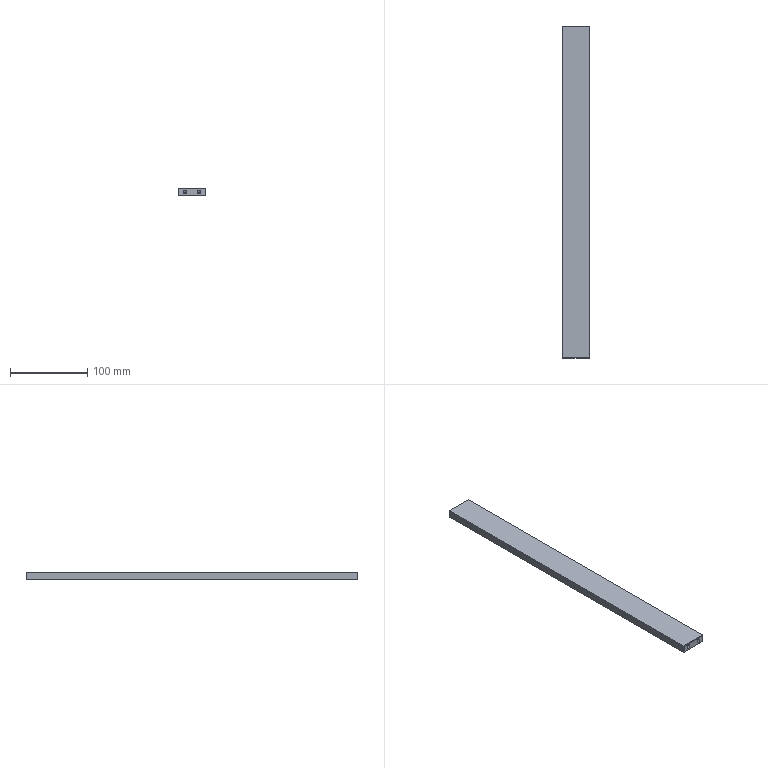Part | STEP file | Pino extrator - Torre - 1 cav | 1 solid | 18 faces | box 35 x 428.85 x 10 mm | volume 149085 mm3 | plane 10 | cylinder 4 | cone 4 | commonest cylinder face diameters 5 x4
STEP:
#1=CARTESIAN_POINT('',(0.,0.,0.));
#2=DIRECTION('',(0.,0.,1.));
#3=DIRECTION('',(1.,0.,0.));
#4=AXIS2_PLACEMENT_3D('',#1,#2,#3);
#5=CARTESIAN_POINT('',(-9.,25.,-2.5));
#6=VERTEX_POINT('',#5);
#7=CARTESIAN_POINT('',(-9.,0.,-2.5));
#8=VERTEX_POINT('',#7);
#9=CARTESIAN_POINT('',(-9.,0.,-2.5));
#10=DIRECTION('',(0.,-1.,0.));
#11=VECTOR('',#10,1.);
#12=LINE('',#9,#11);
#13=CARTESIAN_POINT('',(-9.,0.,0.));
#14=DIRECTION('',(0.,-1.,0.));
#15=DIRECTION('',(0.,0.,-1.));
#16=AXIS2_PLACEMENT_3D('',#13,#14,#15);
#17=CYLINDRICAL_SURFACE('',#16,2.5);
#18=CARTESIAN_POINT('',(6.283,0.));
#19=DIRECTION('',(0.,1.));
#20=VECTOR('',#19,1.);
#21=LINE('',#18,#20);
#22=(GEOMETRIC_REPRESENTATION_CONTEXT(2)PARAMETRIC_REPRESENTATION_CONTEXT()REPRESENTATION_CONTEXT('',''));
#23=DEFINITIONAL_REPRESENTATION('',(#21),#22);
#24=PCURVE('',#17,#23);
#25=CARTESIAN_POINT('',(-9.,0.,0.));
#26=DIRECTION('',(0.,-1.,0.));
#27=DIRECTION('',(0.,0.,-1.));
#28=AXIS2_PLACEMENT_3D('',#25,#26,#27);
#29=CYLINDRICAL_SURFACE('',#28,2.5);
#30=CARTESIAN_POINT('',(0.,0.));
#31=DIRECTION('',(0.,1.));
#32=VECTOR('',#31,1.);
#33=LINE('',#30,#32);
#34=(GEOMETRIC_REPRESENTATION_CONTEXT(2)PARAMETRIC_REPRESENTATION_CONTEXT()REPRESENTATION_CONTEXT('',''));
#35=DEFINITIONAL_REPRESENTATION('',(#33),#34);
#36=PCURVE('',#29,#35);
#37=SURFACE_CURVE('',#12,(#24,#36),.PCURVE_S1.);
#38=EDGE_CURVE('',#6,#8,#37,.T.);
#39=ORIENTED_EDGE('',*,*,#38,.T.);
#40=CARTESIAN_POINT('',(-9.,0.,2.5));
#41=VERTEX_POINT('',#40);
#42=CARTESIAN_POINT('',(-9.,0.,0.));
#43=DIRECTION('',(0.,-1.,0.));
#44=DIRECTION('',(0.,0.,-1.));
#45=AXIS2_PLACEMENT_3D('',#42,#43,#44);
#46=CIRCLE('',#45,2.5);
#47=CARTESIAN_POINT('',(0.,0.));
#48=DIRECTION('',(1.,0.));
#49=VECTOR('',#48,1.);
#50=LINE('',#47,#49);
#51=(GEOMETRIC_REPRESENTATION_CONTEXT(2)PARAMETRIC_REPRESENTATION_CONTEXT()REPRESENTATION_CONTEXT('',''));
#52=DEFINITIONAL_REPRESENTATION('',(#50),#51);
#53=PCURVE('',#17,#52);
#54=CARTESIAN_POINT('',(0.,0.,0.));
#55=DIRECTION('',(0.,-1.,0.));
#56=DIRECTION('',(0.,0.,-1.));
#57=AXIS2_PLACEMENT_3D('',#54,#55,#56);
#58=PLANE('',#57);
#59=CARTESIAN_POINT('',(0.,-9.));
#60=DIRECTION('',(1.,0.));
#61=AXIS2_PLACEMENT_2D('',#59,#60);
#62=CIRCLE('',#61,2.5);
#63=(GEOMETRIC_REPRESENTATION_CONTEXT(2)PARAMETRIC_REPRESENTATION_CONTEXT()REPRESENTATION_CONTEXT('',''));
#64=DEFINITIONAL_REPRESENTATION('',(#62),#63);
#65=PCURVE('',#58,#64);
#66=SURFACE_CURVE('',#46,(#53,#65),.PCURVE_S1.);
#67=EDGE_CURVE('',#41,#8,#66,.T.);
#68=ORIENTED_EDGE('',*,*,#67,.F.);
#69=CARTESIAN_POINT('',(-9.,25.,2.5));
#70=VERTEX_POINT('',#69);
#71=CARTESIAN_POINT('',(-9.,0.,2.5));
#72=DIRECTION('',(0.,-1.,0.));
#73=VECTOR('',#72,1.);
#74=LINE('',#71,#73);
#75=CARTESIAN_POINT('',(3.142,0.));
#76=DIRECTION('',(0.,1.));
#77=VECTOR('',#76,1.);
#78=LINE('',#75,#77);
#79=(GEOMETRIC_REPRESENTATION_CONTEXT(2)PARAMETRIC_REPRESENTATION_CONTEXT()REPRESENTATION_CONTEXT('',''));
#80=DEFINITIONAL_REPRESENTATION('',(#78),#79);
#81=PCURVE('',#17,#80);
#82=CARTESIAN_POINT('',(3.142,0.));
#83=DIRECTION('',(0.,1.));
#84=VECTOR('',#83,1.);
#85=LINE('',#82,#84);
#86=(GEOMETRIC_REPRESENTATION_CONTEXT(2)PARAMETRIC_REPRESENTATION_CONTEXT()REPRESENTATION_CONTEXT('',''));
#87=DEFINITIONAL_REPRESENTATION('',(#85),#86);
#88=PCURVE('',#29,#87);
#89=SURFACE_CURVE('',#74,(#81,#88),.PCURVE_S1.);
#90=EDGE_CURVE('',#70,#41,#89,.T.);
#91=ORIENTED_EDGE('',*,*,#90,.F.);
#92=CARTESIAN_POINT('',(-9.,25.,0.));
#93=DIRECTION('',(0.,-1.,0.));
#94=DIRECTION('',(0.,0.,-1.));
#95=AXIS2_PLACEMENT_3D('',#92,#93,#94);
#96=CIRCLE('',#95,2.5);
#97=CARTESIAN_POINT('',(0.,-25.));
#98=DIRECTION('',(1.,0.));
#99=VECTOR('',#98,1.);
#100=LINE('',#97,#99);
#101=(GEOMETRIC_REPRESENTATION_CONTEXT(2)PARAMETRIC_REPRESENTATION_CONTEXT()REPRESENTATION_CONTEXT('',''));
#102=DEFINITIONAL_REPRESENTATION('',(#100),#101);
#103=PCURVE('',#17,#102);
#104=CARTESIAN_POINT('',(-9.,25.,0.));
#105=DIRECTION('',(0.,-1.,0.));
#106=DIRECTION('',(0.,0.,-1.));
#107=AXIS2_PLACEMENT_3D('',#104,#105,#106);
#108=CONICAL_SURFACE('',#107,2.5,1.03);
#109=CARTESIAN_POINT('',(0.,0.));
#110=DIRECTION('',(1.,0.));
#111=VECTOR('',#110,1.);
#112=LINE('',#109,#111);
#113=(GEOMETRIC_REPRESENTATION_CONTEXT(2)PARAMETRIC_REPRESENTATION_CONTEXT()REPRESENTATION_CONTEXT('',''));
#114=DEFINITIONAL_REPRESENTATION('',(#112),#113);
#115=PCURVE('',#108,#114);
#116=SURFACE_CURVE('',#96,(#103,#115),.PCURVE_S1.);
#117=EDGE_CURVE('',#70,#6,#116,.T.);
#118=ORIENTED_EDGE('',*,*,#117,.T.);
#119=EDGE_LOOP('',(#39,#68,#91,#118));
#120=FACE_BOUND('',#119,.F.);
#121=ADVANCED_FACE('',(#120),#17,.F.);
#122=ORIENTED_EDGE('',*,*,#117,.F.);
#123=CARTESIAN_POINT('',(-9.,26.502,0.));
#124=VERTEX_POINT('',#123);
#125=CARTESIAN_POINT('',(-9.,25.,2.5));
#126=DIRECTION('',(0.,-0.515,0.8572));
#127=VECTOR('',#126,1.);
#128=LINE('',#125,#127);
#129=CARTESIAN_POINT('',(3.142,0.));
#130=DIRECTION('',(0.,1.));
#131=VECTOR('',#130,1.);
#132=LINE('',#129,#131);
#133=(GEOMETRIC_REPRESENTATION_CONTEXT(2)PARAMETRIC_REPRESENTATION_CONTEXT()REPRESENTATION_CONTEXT('',''));
#134=DEFINITIONAL_REPRESENTATION('',(#132),#133);
#135=PCURVE('',#108,#134);
#136=CARTESIAN_POINT('',(-9.,25.,0.));
#137=DIRECTION('',(0.,-1.,0.));
#138=DIRECTION('',(0.,0.,-1.));
#139=AXIS2_PLACEMENT_3D('',#136,#137,#138);
#140=CONICAL_SURFACE('',#139,2.5,1.03);
#141=CARTESIAN_POINT('',(3.142,0.));
#142=DIRECTION('',(0.,1.));
#143=VECTOR('',#142,1.);
#144=LINE('',#141,#143);
#145=(GEOMETRIC_REPRESENTATION_CONTEXT(2)PARAMETRIC_REPRESENTATION_CONTEXT()REPRESENTATION_CONTEXT('',''));
#146=DEFINITIONAL_REPRESENTATION('',(#144),#145);
#147=PCURVE('',#140,#146);
#148=SURFACE_CURVE('',#128,(#135,#147),.PCURVE_S1.);
#149=EDGE_CURVE('',#124,#70,#148,.T.);
#150=ORIENTED_EDGE('',*,*,#149,.F.);
#151=CARTESIAN_POINT('',(-9.,25.,-2.5));
#152=DIRECTION('',(0.,-0.515,-0.8572));
#153=VECTOR('',#152,1.);
#154=LINE('',#151,#153);
#155=CARTESIAN_POINT('',(6.283,0.));
#156=DIRECTION('',(0.,1.));
#157=VECTOR('',#156,1.);
#158=LINE('',#155,#157);
#159=(GEOMETRIC_REPRESENTATION_CONTEXT(2)PARAMETRIC_REPRESENTATION_CONTEXT()REPRESENTATION_CONTEXT('',''));
#160=DEFINITIONAL_REPRESENTATION('',(#158),#159);
#161=PCURVE('',#108,#160);
#162=CARTESIAN_POINT('',(0.,0.));
#163=DIRECTION('',(0.,1.));
#164=VECTOR('',#163,1.);
#165=LINE('',#162,#164);
#166=(GEOMETRIC_REPRESENTATION_CONTEXT(2)PARAMETRIC_REPRESENTATION_CONTEXT()REPRESENTATION_CONTEXT('',''));
#167=DEFINITIONAL_REPRESENTATION('',(#165),#166);
#168=PCURVE('',#140,#167);
#169=SURFACE_CURVE('',#154,(#161,#168),.PCURVE_S1.);
#170=EDGE_CURVE('',#124,#6,#169,.T.);
#171=ORIENTED_EDGE('',*,*,#170,.T.);
#172=EDGE_LOOP('',(#122,#150,#171));
#173=FACE_BOUND('',#172,.F.);
#174=ADVANCED_FACE('',(#173),#108,.F.);
#175=CARTESIAN_POINT('',(9.,25.,-2.5));
#176=VERTEX_POINT('',#175);
#177=CARTESIAN_POINT('',(9.,0.,-2.5));
#178=VERTEX_POINT('',#177);
#179=CARTESIAN_POINT('',(9.,0.,-2.5));
#180=DIRECTION('',(0.,-1.,0.));
#181=VECTOR('',#180,1.);
#182=LINE('',#179,#181);
#183=CARTESIAN_POINT('',(9.,0.,0.));
#184=DIRECTION('',(0.,-1.,0.));
#185=DIRECTION('',(0.,0.,-1.));
#186=AXIS2_PLACEMENT_3D('',#183,#184,#185);
#187=CYLINDRICAL_SURFACE('',#186,2.5);
#188=CARTESIAN_POINT('',(6.283,0.));
#189=DIRECTION('',(0.,1.));
#190=VECTOR('',#189,1.);
#191=LINE('',#188,#190);
#192=(GEOMETRIC_REPRESENTATION_CONTEXT(2)PARAMETRIC_REPRESENTATION_CONTEXT()REPRESENTATION_CONTEXT('',''));
#193=DEFINITIONAL_REPRESENTATION('',(#191),#192);
#194=PCURVE('',#187,#193);
#195=CARTESIAN_POINT('',(9.,0.,0.));
#196=DIRECTION('',(0.,-1.,0.));
#197=DIRECTION('',(0.,0.,-1.));
#198=AXIS2_PLACEMENT_3D('',#195,#196,#197);
#199=CYLINDRICAL_SURFACE('',#198,2.5);
#200=CARTESIAN_POINT('',(0.,0.));
#201=DIRECTION('',(0.,1.));
#202=VECTOR('',#201,1.);
#203=LINE('',#200,#202);
#204=(GEOMETRIC_REPRESENTATION_CONTEXT(2)PARAMETRIC_REPRESENTATION_CONTEXT()REPRESENTATION_CONTEXT('',''));
#205=DEFINITIONAL_REPRESENTATION('',(#203),#204);
#206=PCURVE('',#199,#205);
#207=SURFACE_CURVE('',#182,(#194,#206),.PCURVE_S1.);
#208=EDGE_CURVE('',#176,#178,#207,.T.);
#209=ORIENTED_EDGE('',*,*,#208,.T.);
#210=CARTESIAN_POINT('',(9.,0.,2.5));
#211=VERTEX_POINT('',#210);
#212=CARTESIAN_POINT('',(9.,0.,0.));
#213=DIRECTION('',(0.,-1.,0.));
#214=DIRECTION('',(0.,0.,-1.));
#215=AXIS2_PLACEMENT_3D('',#212,#213,#214);
#216=CIRCLE('',#215,2.5);
#217=CARTESIAN_POINT('',(0.,0.));
#218=DIRECTION('',(1.,0.));
#219=VECTOR('',#218,1.);
#220=LINE('',#217,#219);
#221=(GEOMETRIC_REPRESENTATION_CONTEXT(2)PARAMETRIC_REPRESENTATION_CONTEXT()REPRESENTATION_CONTEXT('',''));
#222=DEFINITIONAL_REPRESENTATION('',(#220),#221);
#223=PCURVE('',#187,#222);
#224=CARTESIAN_POINT('',(0.,9.));
#225=DIRECTION('',(1.,0.));
#226=AXIS2_PLACEMENT_2D('',#224,#225);
#227=CIRCLE('',#226,2.5);
#228=(GEOMETRIC_REPRESENTATION_CONTEXT(2)PARAMETRIC_REPRESENTATION_CONTEXT()REPRESENTATION_CONTEXT('',''));
#229=DEFINITIONAL_REPRESENTATION('',(#227),#228);
#230=PCURVE('',#58,#229);
#231=SURFACE_CURVE('',#216,(#223,#230),.PCURVE_S1.);
#232=EDGE_CURVE('',#211,#178,#231,.T.);
#233=ORIENTED_EDGE('',*,*,#232,.F.);
#234=CARTESIAN_POINT('',(9.,25.,2.5));
#235=VERTEX_POINT('',#234);
#236=CARTESIAN_POINT('',(9.,0.,2.5));
#237=DIRECTION('',(0.,-1.,0.));
#238=VECTOR('',#237,1.);
#239=LINE('',#236,#238);
#240=CARTESIAN_POINT('',(3.142,0.));
#241=DIRECTION('',(0.,1.));
#242=VECTOR('',#241,1.);
#243=LINE('',#240,#242);
#244=(GEOMETRIC_REPRESENTATION_CONTEXT(2)PARAMETRIC_REPRESENTATION_CONTEXT()REPRESENTATION_CONTEXT('',''));
#245=DEFINITIONAL_REPRESENTATION('',(#243),#244);
#246=PCURVE('',#187,#245);
#247=CARTESIAN_POINT('',(3.142,0.));
#248=DIRECTION('',(0.,1.));
#249=VECTOR('',#248,1.);
#250=LINE('',#247,#249);
#251=(GEOMETRIC_REPRESENTATION_CONTEXT(2)PARAMETRIC_REPRESENTATION_CONTEXT()REPRESENTATION_CONTEXT('',''));
#252=DEFINITIONAL_REPRESENTATION('',(#250),#251);
#253=PCURVE('',#199,#252);
#254=SURFACE_CURVE('',#239,(#246,#253),.PCURVE_S1.);
#255=EDGE_CURVE('',#235,#211,#254,.T.);
#256=ORIENTED_EDGE('',*,*,#255,.F.);
#257=CARTESIAN_POINT('',(9.,25.,0.));
#258=DIRECTION('',(0.,-1.,0.));
#259=DIRECTION('',(0.,0.,-1.));
#260=AXIS2_PLACEMENT_3D('',#257,#258,#259);
#261=CIRCLE('',#260,2.5);
#262=CARTESIAN_POINT('',(0.,-25.));
#263=DIRECTION('',(1.,0.));
#264=VECTOR('',#263,1.);
#265=LINE('',#262,#264);
#266=(GEOMETRIC_REPRESENTATION_CONTEXT(2)PARAMETRIC_REPRESENTATION_CONTEXT()REPRESENTATION_CONTEXT('',''));
#267=DEFINITIONAL_REPRESENTATION('',(#265),#266);
#268=PCURVE('',#187,#267);
#269=CARTESIAN_POINT('',(9.,25.,0.));
#270=DIRECTION('',(0.,-1.,0.));
#271=DIRECTION('',(0.,0.,-1.));
#272=AXIS2_PLACEMENT_3D('',#269,#270,#271);
#273=CONICAL_SURFACE('',#272,2.5,1.03);
#274=CARTESIAN_POINT('',(0.,0.));
#275=DIRECTION('',(1.,0.));
#276=VECTOR('',#275,1.);
#277=LINE('',#274,#276);
#278=(GEOMETRIC_REPRESENTATION_CONTEXT(2)PARAMETRIC_REPRESENTATION_CONTEXT()REPRESENTATION_CONTEXT('',''));
#279=DEFINITIONAL_REPRESENTATION('',(#277),#278);
#280=PCURVE('',#273,#279);
#281=SURFACE_CURVE('',#261,(#268,#280),.PCURVE_S1.);
#282=EDGE_CURVE('',#235,#176,#281,.T.);
#283=ORIENTED_EDGE('',*,*,#282,.T.);
#284=EDGE_LOOP('',(#209,#233,#256,#283));
#285=FACE_BOUND('',#284,.F.);
#286=ADVANCED_FACE('',(#285),#187,.F.);
#287=ORIENTED_EDGE('',*,*,#282,.F.);
#288=CARTESIAN_POINT('',(9.,26.502,0.));
#289=VERTEX_POINT('',#288);
#290=CARTESIAN_POINT('',(9.,25.,2.5));
#291=DIRECTION('',(0.,-0.515,0.8572));
#292=VECTOR('',#291,1.);
#293=LINE('',#290,#292);
#294=CARTESIAN_POINT('',(3.142,0.));
#295=DIRECTION('',(0.,1.));
#296=VECTOR('',#295,1.);
#297=LINE('',#294,#296);
#298=(GEOMETRIC_REPRESENTATION_CONTEXT(2)PARAMETRIC_REPRESENTATION_CONTEXT()REPRESENTATION_CONTEXT('',''));
#299=DEFINITIONAL_REPRESENTATION('',(#297),#298);
#300=PCURVE('',#273,#299);
#301=CARTESIAN_POINT('',(9.,25.,0.));
#302=DIRECTION('',(0.,-1.,0.));
#303=DIRECTION('',(0.,0.,-1.));
#304=AXIS2_PLACEMENT_3D('',#301,#302,#303);
#305=CONICAL_SURFACE('',#304,2.5,1.03);
#306=CARTESIAN_POINT('',(3.142,0.));
#307=DIRECTION('',(0.,1.));
#308=VECTOR('',#307,1.);
#309=LINE('',#306,#308);
#310=(GEOMETRIC_REPRESENTATION_CONTEXT(2)PARAMETRIC_REPRESENTATION_CONTEXT()REPRESENTATION_CONTEXT('',''));
#311=DEFINITIONAL_REPRESENTATION('',(#309),#310);
#312=PCURVE('',#305,#311);
#313=SURFACE_CURVE('',#293,(#300,#312),.PCURVE_S1.);
#314=EDGE_CURVE('',#289,#235,#313,.T.);
#315=ORIENTED_EDGE('',*,*,#314,.F.);
#316=CARTESIAN_POINT('',(9.,25.,-2.5));
#317=DIRECTION('',(0.,-0.515,-0.8572));
#318=VECTOR('',#317,1.);
#319=LINE('',#316,#318);
#320=CARTESIAN_POINT('',(6.283,0.));
#321=DIRECTION('',(0.,1.));
#322=VECTOR('',#321,1.);
#323=LINE('',#320,#322);
#324=(GEOMETRIC_REPRESENTATION_CONTEXT(2)PARAMETRIC_REPRESENTATION_CONTEXT()REPRESENTATION_CONTEXT('',''));
#325=DEFINITIONAL_REPRESENTATION('',(#323),#324);
#326=PCURVE('',#273,#325);
#327=CARTESIAN_POINT('',(0.,0.));
#328=DIRECTION('',(0.,1.));
#329=VECTOR('',#328,1.);
#330=LINE('',#327,#329);
#331=(GEOMETRIC_REPRESENTATION_CONTEXT(2)PARAMETRIC_REPRESENTATION_CONTEXT()REPRESENTATION_CONTEXT('',''));
#332=DEFINITIONAL_REPRESENTATION('',(#330),#331);
#333=PCURVE('',#305,#332);
#334=SURFACE_CURVE('',#319,(#326,#333),.PCURVE_S1.);
#335=EDGE_CURVE('',#289,#176,#334,.T.);
#336=ORIENTED_EDGE('',*,*,#335,.T.);
#337=EDGE_LOOP('',(#287,#315,#336));
#338=FACE_BOUND('',#337,.F.);
#339=ADVANCED_FACE('',(#338),#273,.F.);
#340=CARTESIAN_POINT('',(17.5,428.85,5.));
#341=VERTEX_POINT('',#340);
#342=CARTESIAN_POINT('',(17.5,0.5,5.));
#343=VERTEX_POINT('',#342);
#344=CARTESIAN_POINT('',(17.5,428.85,5.));
#345=DIRECTION('',(0.,-1.,0.));
#346=VECTOR('',#345,1.);
#347=LINE('',#344,#346);
#348=CARTESIAN_POINT('',(17.5,428.85,5.));
#349=DIRECTION('',(-1.,0.,0.));
#350=DIRECTION('',(0.,0.,1.));
#351=AXIS2_PLACEMENT_3D('',#348,#349,#350);
#352=PLANE('',#351);
#353=CARTESIAN_POINT('',(0.,0.));
#354=DIRECTION('',(0.,-1.));
#355=VECTOR('',#354,1.);
#356=LINE('',#353,#355);
#357=(GEOMETRIC_REPRESENTATION_CONTEXT(2)PARAMETRIC_REPRESENTATION_CONTEXT()REPRESENTATION_CONTEXT('',''));
#358=DEFINITIONAL_REPRESENTATION('',(#356),#357);
#359=PCURVE('',#352,#358);
#360=CARTESIAN_POINT('',(-17.5,428.85,5.));
#361=DIRECTION('',(0.,0.,-1.));
#362=DIRECTION('',(-1.,0.,0.));
#363=AXIS2_PLACEMENT_3D('',#360,#361,#362);
#364=PLANE('',#363);
#365=CARTESIAN_POINT('',(-35.,0.));
#366=DIRECTION('',(0.,-1.));
#367=VECTOR('',#366,1.);
#368=LINE('',#365,#367);
#369=(GEOMETRIC_REPRESENTATION_CONTEXT(2)PARAMETRIC_REPRESENTATION_CONTEXT()REPRESENTATION_CONTEXT('',''));
#370=DEFINITIONAL_REPRESENTATION('',(#368),#369);
#371=PCURVE('',#364,#370);
#372=SURFACE_CURVE('',#347,(#359,#371),.PCURVE_S1.);
#373=EDGE_CURVE('',#341,#343,#372,.T.);
#374=ORIENTED_EDGE('',*,*,#373,.T.);
#375=CARTESIAN_POINT('',(17.5,0.5,-5.));
#376=VERTEX_POINT('',#375);
#377=CARTESIAN_POINT('',(17.5,0.5,-5.));
#378=DIRECTION('',(0.,0.,-1.));
#379=VECTOR('',#378,1.);
#380=LINE('',#377,#379);
#381=CARTESIAN_POINT('',(-10.,-428.35));
#382=DIRECTION('',(-1.,0.));
#383=VECTOR('',#382,1.);
#384=LINE('',#381,#383);
#385=(GEOMETRIC_REPRESENTATION_CONTEXT(2)PARAMETRIC_REPRESENTATION_CONTEXT()REPRESENTATION_CONTEXT('',''));
#386=DEFINITIONAL_REPRESENTATION('',(#384),#385);
#387=PCURVE('',#352,#386);
#388=CARTESIAN_POINT('',(17.5,0.5,5.));
#389=DIRECTION('',(0.7071,-0.7071,0.));
#390=DIRECTION('',(0.,0.,1.));
#391=AXIS2_PLACEMENT_3D('',#388,#389,#390);
#392=PLANE('',#391);
#393=CARTESIAN_POINT('',(-10.,0.));
#394=DIRECTION('',(-1.,0.));
#395=VECTOR('',#394,1.);
#396=LINE('',#393,#395);
#397=(GEOMETRIC_REPRESENTATION_CONTEXT(2)PARAMETRIC_REPRESENTATION_CONTEXT()REPRESENTATION_CONTEXT('',''));
#398=DEFINITIONAL_REPRESENTATION('',(#396),#397);
#399=PCURVE('',#392,#398);
#400=SURFACE_CURVE('',#380,(#387,#399),.PCURVE_S1.);
#401=EDGE_CURVE('',#343,#376,#400,.T.);
#402=ORIENTED_EDGE('',*,*,#401,.T.);
#403=CARTESIAN_POINT('',(17.5,428.85,-5.));
#404=VERTEX_POINT('',#403);
#405=CARTESIAN_POINT('',(17.5,428.85,-5.));
#406=DIRECTION('',(0.,-1.,0.));
#407=VECTOR('',#406,1.);
#408=LINE('',#405,#407);
#409=CARTESIAN_POINT('',(-10.,0.));
#410=DIRECTION('',(0.,-1.));
#411=VECTOR('',#410,1.);
#412=LINE('',#409,#411);
#413=(GEOMETRIC_REPRESENTATION_CONTEXT(2)PARAMETRIC_REPRESENTATION_CONTEXT()REPRESENTATION_CONTEXT('',''));
#414=DEFINITIONAL_REPRESENTATION('',(#412),#413);
#415=PCURVE('',#352,#414);
#416=CARTESIAN_POINT('',(-17.5,428.85,-5.));
#417=DIRECTION('',(0.,0.,1.));
#418=DIRECTION('',(1.,0.,0.));
#419=AXIS2_PLACEMENT_3D('',#416,#417,#418);
#420=PLANE('',#419);
#421=CARTESIAN_POINT('',(35.,0.));
#422=DIRECTION('',(0.,-1.));
#423=VECTOR('',#422,1.);
#424=LINE('',#421,#423);
#425=(GEOMETRIC_REPRESENTATION_CONTEXT(2)PARAMETRIC_REPRESENTATION_CONTEXT()REPRESENTATION_CONTEXT('',''));
#426=DEFINITIONAL_REPRESENTATION('',(#424),#425);
#427=PCURVE('',#420,#426);
#428=SURFACE_CURVE('',#408,(#415,#427),.PCURVE_S1.);
#429=EDGE_CURVE('',#404,#376,#428,.T.);
#430=ORIENTED_EDGE('',*,*,#429,.F.);
#431=CARTESIAN_POINT('',(17.5,428.85,5.));
#432=DIRECTION('',(0.,0.,-1.));
#433=VECTOR('',#432,1.);
#434=LINE('',#431,#433);
#435=CARTESIAN_POINT('',(0.,0.));
#436=DIRECTION('',(-1.,0.));
#437=VECTOR('',#436,1.);
#438=LINE('',#435,#437);
#439=(GEOMETRIC_REPRESENTATION_CONTEXT(2)PARAMETRIC_REPRESENTATION_CONTEXT()REPRESENTATION_CONTEXT('',''));
#440=DEFINITIONAL_REPRESENTATION('',(#438),#439);
#441=PCURVE('',#352,#440);
#442=CARTESIAN_POINT('',(0.,428.85,0.));
#443=DIRECTION('',(0.,-1.,0.));
#444=DIRECTION('',(0.,0.,-1.));
#445=AXIS2_PLACEMENT_3D('',#442,#443,#444);
#446=PLANE('',#445);
#447=CARTESIAN_POINT('',(-5.,17.5));
#448=DIRECTION('',(1.,0.));
#449=VECTOR('',#448,1.);
#450=LINE('',#447,#449);
#451=(GEOMETRIC_REPRESENTATION_CONTEXT(2)PARAMETRIC_REPRESENTATION_CONTEXT()REPRESENTATION_CONTEXT('',''));
#452=DEFINITIONAL_REPRESENTATION('',(#450),#451);
#453=PCURVE('',#446,#452);
#454=SURFACE_CURVE('',#434,(#441,#453),.PCURVE_S1.);
#455=EDGE_CURVE('',#341,#404,#454,.T.);
#456=ORIENTED_EDGE('',*,*,#455,.F.);
#457=EDGE_LOOP('',(#374,#402,#430,#456));
#458=FACE_BOUND('',#457,.T.);
#459=ADVANCED_FACE('',(#458),#352,.F.);
#460=ORIENTED_EDGE('',*,*,#429,.T.);
#461=CARTESIAN_POINT('',(-17.5,0.5,-5.));
#462=VERTEX_POINT('',#461);
#463=CARTESIAN_POINT('',(-17.5,0.5,-5.));
#464=DIRECTION('',(-1.,0.,0.));
#465=VECTOR('',#464,1.);
#466=LINE('',#463,#465);
#467=CARTESIAN_POINT('',(0.,-428.35));
#468=DIRECTION('',(-1.,0.));
#469=VECTOR('',#468,1.);
#470=LINE('',#467,#469);
#471=(GEOMETRIC_REPRESENTATION_CONTEXT(2)PARAMETRIC_REPRESENTATION_CONTEXT()REPRESENTATION_CONTEXT('',''));
#472=DEFINITIONAL_REPRESENTATION('',(#470),#471);
#473=PCURVE('',#420,#472);
#474=CARTESIAN_POINT('',(-17.5,0.5,-5.));
#475=DIRECTION('',(0.,-0.7071,-0.7071));
#476=DIRECTION('',(1.,0.,0.));
#477=AXIS2_PLACEMENT_3D('',#474,#475,#476);
#478=PLANE('',#477);
#479=CARTESIAN_POINT('',(0.,0.));
#480=DIRECTION('',(-1.,0.));
#481=VECTOR('',#480,1.);
#482=LINE('',#479,#481);
#483=(GEOMETRIC_REPRESENTATION_CONTEXT(2)PARAMETRIC_REPRESENTATION_CONTEXT()REPRESENTATION_CONTEXT('',''));
#484=DEFINITIONAL_REPRESENTATION('',(#482),#483);
#485=PCURVE('',#478,#484);
#486=SURFACE_CURVE('',#466,(#473,#485),.PCURVE_S1.);
#487=EDGE_CURVE('',#376,#462,#486,.T.);
#488=ORIENTED_EDGE('',*,*,#487,.T.);
#489=CARTESIAN_POINT('',(-17.5,428.85,-5.));
#490=VERTEX_POINT('',#489);
#491=CARTESIAN_POINT('',(-17.5,428.85,-5.));
#492=DIRECTION('',(0.,-1.,0.));
#493=VECTOR('',#492,1.);
#494=LINE('',#491,#493);
#495=CARTESIAN_POINT('',(0.,0.));
#496=DIRECTION('',(0.,-1.));
#497=VECTOR('',#496,1.);
#498=LINE('',#495,#497);
#499=(GEOMETRIC_REPRESENTATION_CONTEXT(2)PARAMETRIC_REPRESENTATION_CONTEXT()REPRESENTATION_CONTEXT('',''));
#500=DEFINITIONAL_REPRESENTATION('',(#498),#499);
#501=PCURVE('',#420,#500);
#502=CARTESIAN_POINT('',(-17.5,428.85,5.));
#503=DIRECTION('',(1.,0.,0.));
#504=DIRECTION('',(0.,0.,-1.));
#505=AXIS2_PLACEMENT_3D('',#502,#503,#504);
#506=PLANE('',#505);
#507=CARTESIAN_POINT('',(10.,0.));
#508=DIRECTION('',(0.,-1.));
#509=VECTOR('',#508,1.);
#510=LINE('',#507,#509);
#511=(GEOMETRIC_REPRESENTATION_CONTEXT(2)PARAMETRIC_REPRESENTATION_CONTEXT()REPRESENTATION_CONTEXT('',''));
#512=DEFINITIONAL_REPRESENTATION('',(#510),#511);
#513=PCURVE('',#506,#512);
#514=SURFACE_CURVE('',#494,(#501,#513),.PCURVE_S1.);
#515=EDGE_CURVE('',#490,#462,#514,.T.);
#516=ORIENTED_EDGE('',*,*,#515,.F.);
#517=CARTESIAN_POINT('',(-17.5,428.85,-5.));
#518=DIRECTION('',(-1.,0.,0.));
#519=VECTOR('',#518,1.);
#520=LINE('',#517,#519);
#521=CARTESIAN_POINT('',(0.,0.));
#522=DIRECTION('',(-1.,0.));
#523=VECTOR('',#522,1.);
#524=LINE('',#521,#523);
#525=(GEOMETRIC_REPRESENTATION_CONTEXT(2)PARAMETRIC_REPRESENTATION_CONTEXT()REPRESENTATION_CONTEXT('',''));
#526=DEFINITIONAL_REPRESENTATION('',(#524),#525);
#527=PCURVE('',#420,#526);
#528=CARTESIAN_POINT('',(5.,-17.5));
#529=DIRECTION('',(0.,-1.));
#530=VECTOR('',#529,1.);
#531=LINE('',#528,#530);
#532=(GEOMETRIC_REPRESENTATION_CONTEXT(2)PARAMETRIC_REPRESENTATION_CONTEXT()REPRESENTATION_CONTEXT('',''));
#533=DEFINITIONAL_REPRESENTATION('',(#531),#532);
#534=PCURVE('',#446,#533);
#535=SURFACE_CURVE('',#520,(#527,#534),.PCURVE_S1.);
#536=EDGE_CURVE('',#404,#490,#535,.T.);
#537=ORIENTED_EDGE('',*,*,#536,.F.);
#538=EDGE_LOOP('',(#460,#488,#516,#537));
#539=FACE_BOUND('',#538,.T.);
#540=ADVANCED_FACE('',(#539),#420,.F.);
#541=ORIENTED_EDGE('',*,*,#515,.T.);
#542=CARTESIAN_POINT('',(-17.5,0.5,5.));
#543=VERTEX_POINT('',#542);
#544=CARTESIAN_POINT('',(-17.5,0.5,5.));
#545=DIRECTION('',(0.,0.,1.));
#546=VECTOR('',#545,1.);
#547=LINE('',#544,#546);
#548=CARTESIAN_POINT('',(0.,-428.35));
#549=DIRECTION('',(-1.,0.));
#550=VECTOR('',#549,1.);
#551=LINE('',#548,#550);
#552=(GEOMETRIC_REPRESENTATION_CONTEXT(2)PARAMETRIC_REPRESENTATION_CONTEXT()REPRESENTATION_CONTEXT('',''));
#553=DEFINITIONAL_REPRESENTATION('',(#551),#552);
#554=PCURVE('',#506,#553);
#555=CARTESIAN_POINT('',(-17.5,0.5,5.));
#556=DIRECTION('',(-0.7071,-0.7071,0.));
#557=DIRECTION('',(0.,0.,-1.));
#558=AXIS2_PLACEMENT_3D('',#555,#556,#557);
#559=PLANE('',#558);
#560=CARTESIAN_POINT('',(0.,0.));
#561=DIRECTION('',(-1.,0.));
#562=VECTOR('',#561,1.);
#563=LINE('',#560,#562);
#564=(GEOMETRIC_REPRESENTATION_CONTEXT(2)PARAMETRIC_REPRESENTATION_CONTEXT()REPRESENTATION_CONTEXT('',''));
#565=DEFINITIONAL_REPRESENTATION('',(#563),#564);
#566=PCURVE('',#559,#565);
#567=SURFACE_CURVE('',#547,(#554,#566),.PCURVE_S1.);
#568=EDGE_CURVE('',#462,#543,#567,.T.);
#569=ORIENTED_EDGE('',*,*,#568,.T.);
#570=CARTESIAN_POINT('',(-17.5,428.85,5.));
#571=VERTEX_POINT('',#570);
#572=CARTESIAN_POINT('',(-17.5,428.85,5.));
#573=DIRECTION('',(0.,-1.,0.));
#574=VECTOR('',#573,1.);
#575=LINE('',#572,#574);
#576=CARTESIAN_POINT('',(0.,0.));
#577=DIRECTION('',(0.,-1.));
#578=VECTOR('',#577,1.);
#579=LINE('',#576,#578);
#580=(GEOMETRIC_REPRESENTATION_CONTEXT(2)PARAMETRIC_REPRESENTATION_CONTEXT()REPRESENTATION_CONTEXT('',''));
#581=DEFINITIONAL_REPRESENTATION('',(#579),#580);
#582=PCURVE('',#506,#581);
#583=CARTESIAN_POINT('',(0.,0.));
#584=DIRECTION('',(0.,-1.));
#585=VECTOR('',#584,1.);
#586=LINE('',#583,#585);
#587=(GEOMETRIC_REPRESENTATION_CONTEXT(2)PARAMETRIC_REPRESENTATION_CONTEXT()REPRESENTATION_CONTEXT('',''));
#588=DEFINITIONAL_REPRESENTATION('',(#586),#587);
#589=PCURVE('',#364,#588);
#590=SURFACE_CURVE('',#575,(#582,#589),.PCURVE_S1.);
#591=EDGE_CURVE('',#571,#543,#590,.T.);
#592=ORIENTED_EDGE('',*,*,#591,.F.);
#593=CARTESIAN_POINT('',(-17.5,428.85,5.));
#594=DIRECTION('',(0.,0.,1.));
#595=VECTOR('',#594,1.);
#596=LINE('',#593,#595);
#597=CARTESIAN_POINT('',(0.,0.));
#598=DIRECTION('',(-1.,0.));
#599=VECTOR('',#598,1.);
#600=LINE('',#597,#599);
#601=(GEOMETRIC_REPRESENTATION_CONTEXT(2)PARAMETRIC_REPRESENTATION_CONTEXT()REPRESENTATION_CONTEXT('',''));
#602=DEFINITIONAL_REPRESENTATION('',(#600),#601);
#603=PCURVE('',#506,#602);
#604=CARTESIAN_POINT('',(-5.,-17.5));
#605=DIRECTION('',(-1.,0.));
#606=VECTOR('',#605,1.);
#607=LINE('',#604,#606);
#608=(GEOMETRIC_REPRESENTATION_CONTEXT(2)PARAMETRIC_REPRESENTATION_CONTEXT()REPRESENTATION_CONTEXT('',''));
#609=DEFINITIONAL_REPRESENTATION('',(#607),#608);
#610=PCURVE('',#446,#609);
#611=SURFACE_CURVE('',#596,(#603,#610),.PCURVE_S1.);
#612=EDGE_CURVE('',#490,#571,#611,.T.);
#613=ORIENTED_EDGE('',*,*,#612,.F.);
#614=EDGE_LOOP('',(#541,#569,#592,#613));
#615=FACE_BOUND('',#614,.T.);
#616=ADVANCED_FACE('',(#615),#506,.F.);
#617=ORIENTED_EDGE('',*,*,#591,.T.);
#618=CARTESIAN_POINT('',(17.5,0.5,5.));
#619=DIRECTION('',(1.,0.,0.));
#620=VECTOR('',#619,1.);
#621=LINE('',#618,#620);
#622=CARTESIAN_POINT('',(-35.,-428.35));
#623=DIRECTION('',(-1.,0.));
#624=VECTOR('',#623,1.);
#625=LINE('',#622,#624);
#626=(GEOMETRIC_REPRESENTATION_CONTEXT(2)PARAMETRIC_REPRESENTATION_CONTEXT()REPRESENTATION_CONTEXT('',''));
#627=DEFINITIONAL_REPRESENTATION('',(#625),#626);
#628=PCURVE('',#364,#627);
#629=CARTESIAN_POINT('',(-17.5,0.5,5.));
#630=DIRECTION('',(0.,-0.7071,0.7071));
#631=DIRECTION('',(-1.,0.,0.));
#632=AXIS2_PLACEMENT_3D('',#629,#630,#631);
#633=PLANE('',#632);
#634=CARTESIAN_POINT('',(-35.,0.));
#635=DIRECTION('',(-1.,0.));
#636=VECTOR('',#635,1.);
#637=LINE('',#634,#636);
#638=(GEOMETRIC_REPRESENTATION_CONTEXT(2)PARAMETRIC_REPRESENTATION_CONTEXT()REPRESENTATION_CONTEXT('',''));
#639=DEFINITIONAL_REPRESENTATION('',(#637),#638);
#640=PCURVE('',#633,#639);
#641=SURFACE_CURVE('',#621,(#628,#640),.PCURVE_S1.);
#642=EDGE_CURVE('',#543,#343,#641,.T.);
#643=ORIENTED_EDGE('',*,*,#642,.T.);
#644=ORIENTED_EDGE('',*,*,#373,.F.);
#645=CARTESIAN_POINT('',(-17.5,428.85,5.));
#646=DIRECTION('',(1.,0.,0.));
#647=VECTOR('',#646,1.);
#648=LINE('',#645,#647);
#649=CARTESIAN_POINT('',(0.,0.));
#650=DIRECTION('',(-1.,0.));
#651=VECTOR('',#650,1.);
#652=LINE('',#649,#651);
#653=(GEOMETRIC_REPRESENTATION_CONTEXT(2)PARAMETRIC_REPRESENTATION_CONTEXT()REPRESENTATION_CONTEXT('',''));
#654=DEFINITIONAL_REPRESENTATION('',(#652),#653);
#655=PCURVE('',#364,#654);
#656=CARTESIAN_POINT('',(-5.,-17.5));
#657=DIRECTION('',(0.,1.));
#658=VECTOR('',#657,1.);
#659=LINE('',#656,#658);
#660=(GEOMETRIC_REPRESENTATION_CONTEXT(2)PARAMETRIC_REPRESENTATION_CONTEXT()REPRESENTATION_CONTEXT('',''));
#661=DEFINITIONAL_REPRESENTATION('',(#659),#660);
#662=PCURVE('',#446,#661);
#663=SURFACE_CURVE('',#648,(#655,#662),.PCURVE_S1.);
#664=EDGE_CURVE('',#571,#341,#663,.T.);
#665=ORIENTED_EDGE('',*,*,#664,.F.);
#666=EDGE_LOOP('',(#617,#643,#644,#665));
#667=FACE_BOUND('',#666,.T.);
#668=ADVANCED_FACE('',(#667),#364,.F.);
#669=ORIENTED_EDGE('',*,*,#455,.T.);
#670=ORIENTED_EDGE('',*,*,#536,.T.);
#671=ORIENTED_EDGE('',*,*,#612,.T.);
#672=ORIENTED_EDGE('',*,*,#664,.T.);
#673=EDGE_LOOP('',(#669,#670,#671,#672));
#674=FACE_BOUND('',#673,.T.);
#675=ADVANCED_FACE('',(#674),#446,.F.);
#676=CARTESIAN_POINT('',(17.,0.,4.5));
#677=VERTEX_POINT('',#676);
#678=CARTESIAN_POINT('',(-17.,0.,4.5));
#679=VERTEX_POINT('',#678);
#680=CARTESIAN_POINT('',(-17.5,0.,4.5));
#681=DIRECTION('',(-1.,0.,0.));
#682=VECTOR('',#681,1.);
#683=LINE('',#680,#682);
#684=CARTESIAN_POINT('',(-4.5,-17.5));
#685=DIRECTION('',(0.,-1.));
#686=VECTOR('',#685,1.);
#687=LINE('',#684,#686);
#688=(GEOMETRIC_REPRESENTATION_CONTEXT(2)PARAMETRIC_REPRESENTATION_CONTEXT()REPRESENTATION_CONTEXT('',''));
#689=DEFINITIONAL_REPRESENTATION('',(#687),#688);
#690=PCURVE('',#58,#689);
#691=CARTESIAN_POINT('',(0.,0.7071));
#692=DIRECTION('',(1.,0.));
#693=VECTOR('',#692,1.);
#694=LINE('',#691,#693);
#695=(GEOMETRIC_REPRESENTATION_CONTEXT(2)PARAMETRIC_REPRESENTATION_CONTEXT()REPRESENTATION_CONTEXT('',''));
#696=DEFINITIONAL_REPRESENTATION('',(#694),#695);
#697=PCURVE('',#633,#696);
#698=SURFACE_CURVE('',#683,(#690,#697),.PCURVE_S1.);
#699=EDGE_CURVE('',#677,#679,#698,.T.);
#700=ORIENTED_EDGE('',*,*,#699,.T.);
#701=CARTESIAN_POINT('',(-17.,0.,-4.5));
#702=VERTEX_POINT('',#701);
#703=CARTESIAN_POINT('',(-17.,0.,-5.));
#704=DIRECTION('',(0.,0.,-1.));
#705=VECTOR('',#704,1.);
#706=LINE('',#703,#705);
#707=CARTESIAN_POINT('',(5.,-17.));
#708=DIRECTION('',(1.,0.));
#709=VECTOR('',#708,1.);
#710=LINE('',#707,#709);
#711=(GEOMETRIC_REPRESENTATION_CONTEXT(2)PARAMETRIC_REPRESENTATION_CONTEXT()REPRESENTATION_CONTEXT('',''));
#712=DEFINITIONAL_REPRESENTATION('',(#710),#711);
#713=PCURVE('',#58,#712);
#714=CARTESIAN_POINT('',(10.,0.7071));
#715=DIRECTION('',(1.,0.));
#716=VECTOR('',#715,1.);
#717=LINE('',#714,#716);
#718=(GEOMETRIC_REPRESENTATION_CONTEXT(2)PARAMETRIC_REPRESENTATION_CONTEXT()REPRESENTATION_CONTEXT('',''));
#719=DEFINITIONAL_REPRESENTATION('',(#717),#718);
#720=PCURVE('',#559,#719);
#721=SURFACE_CURVE('',#706,(#713,#720),.PCURVE_S1.);
#722=EDGE_CURVE('',#679,#702,#721,.T.);
#723=ORIENTED_EDGE('',*,*,#722,.T.);
#724=CARTESIAN_POINT('',(17.,0.,-4.5));
#725=VERTEX_POINT('',#724);
#726=CARTESIAN_POINT('',(17.5,0.,-4.5));
#727=DIRECTION('',(1.,0.,0.));
#728=VECTOR('',#727,1.);
#729=LINE('',#726,#728);
#730=CARTESIAN_POINT('',(4.5,17.5));
#731=DIRECTION('',(0.,1.));
#732=VECTOR('',#731,1.);
#733=LINE('',#730,#732);
#734=(GEOMETRIC_REPRESENTATION_CONTEXT(2)PARAMETRIC_REPRESENTATION_CONTEXT()REPRESENTATION_CONTEXT('',''));
#735=DEFINITIONAL_REPRESENTATION('',(#733),#734);
#736=PCURVE('',#58,#735);
#737=CARTESIAN_POINT('',(35.,0.7071));
#738=DIRECTION('',(1.,0.));
#739=VECTOR('',#738,1.);
#740=LINE('',#737,#739);
#741=(GEOMETRIC_REPRESENTATION_CONTEXT(2)PARAMETRIC_REPRESENTATION_CONTEXT()REPRESENTATION_CONTEXT('',''));
#742=DEFINITIONAL_REPRESENTATION('',(#740),#741);
#743=PCURVE('',#478,#742);
#744=SURFACE_CURVE('',#729,(#736,#743),.PCURVE_S1.);
#745=EDGE_CURVE('',#702,#725,#744,.T.);
#746=ORIENTED_EDGE('',*,*,#745,.T.);
#747=CARTESIAN_POINT('',(17.,0.,5.));
#748=DIRECTION('',(0.,0.,1.));
#749=VECTOR('',#748,1.);
#750=LINE('',#747,#749);
#751=CARTESIAN_POINT('',(-5.,17.));
#752=DIRECTION('',(-1.,0.));
#753=VECTOR('',#752,1.);
#754=LINE('',#751,#753);
#755=(GEOMETRIC_REPRESENTATION_CONTEXT(2)PARAMETRIC_REPRESENTATION_CONTEXT()REPRESENTATION_CONTEXT('',''));
#756=DEFINITIONAL_REPRESENTATION('',(#754),#755);
#757=PCURVE('',#58,#756);
#758=CARTESIAN_POINT('',(0.,0.7071));
#759=DIRECTION('',(1.,0.));
#760=VECTOR('',#759,1.);
#761=LINE('',#758,#760);
#762=(GEOMETRIC_REPRESENTATION_CONTEXT(2)PARAMETRIC_REPRESENTATION_CONTEXT()REPRESENTATION_CONTEXT('',''));
#763=DEFINITIONAL_REPRESENTATION('',(#761),#762);
#764=PCURVE('',#392,#763);
#765=SURFACE_CURVE('',#750,(#757,#764),.PCURVE_S1.);
#766=EDGE_CURVE('',#725,#677,#765,.T.);
#767=ORIENTED_EDGE('',*,*,#766,.T.);
#768=EDGE_LOOP('',(#700,#723,#746,#767));
#769=FACE_BOUND('',#768,.T.);
#770=CARTESIAN_POINT('',(-9.,0.,0.));
#771=DIRECTION('',(0.,-1.,0.));
#772=DIRECTION('',(0.,0.,-1.));
#773=AXIS2_PLACEMENT_3D('',#770,#771,#772);
#774=CIRCLE('',#773,2.5);
#775=CARTESIAN_POINT('',(0.,-9.));
#776=DIRECTION('',(1.,0.));
#777=AXIS2_PLACEMENT_2D('',#775,#776);
#778=CIRCLE('',#777,2.5);
#779=(GEOMETRIC_REPRESENTATION_CONTEXT(2)PARAMETRIC_REPRESENTATION_CONTEXT()REPRESENTATION_CONTEXT('',''));
#780=DEFINITIONAL_REPRESENTATION('',(#778),#779);
#781=PCURVE('',#58,#780);
#782=CARTESIAN_POINT('',(0.,0.));
#783=DIRECTION('',(1.,0.));
#784=VECTOR('',#783,1.);
#785=LINE('',#782,#784);
#786=(GEOMETRIC_REPRESENTATION_CONTEXT(2)PARAMETRIC_REPRESENTATION_CONTEXT()REPRESENTATION_CONTEXT('',''));
#787=DEFINITIONAL_REPRESENTATION('',(#785),#786);
#788=PCURVE('',#29,#787);
#789=SURFACE_CURVE('',#774,(#781,#788),.PCURVE_S1.);
#790=EDGE_CURVE('',#8,#41,#789,.T.);
#791=ORIENTED_EDGE('',*,*,#790,.F.);
#792=ORIENTED_EDGE('',*,*,#67,.F.);
#793=EDGE_LOOP('',(#791,#792));
#794=FACE_BOUND('',#793,.T.);
#795=CARTESIAN_POINT('',(9.,0.,0.));
#796=DIRECTION('',(0.,-1.,0.));
#797=DIRECTION('',(0.,0.,-1.));
#798=AXIS2_PLACEMENT_3D('',#795,#796,#797);
#799=CIRCLE('',#798,2.5);
#800=CARTESIAN_POINT('',(0.,9.));
#801=DIRECTION('',(1.,0.));
#802=AXIS2_PLACEMENT_2D('',#800,#801);
#803=CIRCLE('',#802,2.5);
#804=(GEOMETRIC_REPRESENTATION_CONTEXT(2)PARAMETRIC_REPRESENTATION_CONTEXT()REPRESENTATION_CONTEXT('',''));
#805=DEFINITIONAL_REPRESENTATION('',(#803),#804);
#806=PCURVE('',#58,#805);
#807=CARTESIAN_POINT('',(0.,0.));
#808=DIRECTION('',(1.,0.));
#809=VECTOR('',#808,1.);
#810=LINE('',#807,#809);
#811=(GEOMETRIC_REPRESENTATION_CONTEXT(2)PARAMETRIC_REPRESENTATION_CONTEXT()REPRESENTATION_CONTEXT('',''));
#812=DEFINITIONAL_REPRESENTATION('',(#810),#811);
#813=PCURVE('',#199,#812);
#814=SURFACE_CURVE('',#799,(#806,#813),.PCURVE_S1.);
#815=EDGE_CURVE('',#178,#211,#814,.T.);
#816=ORIENTED_EDGE('',*,*,#815,.F.);
#817=ORIENTED_EDGE('',*,*,#232,.F.);
#818=EDGE_LOOP('',(#816,#817));
#819=FACE_BOUND('',#818,.T.);
#820=ADVANCED_FACE('',(#769,#794,#819),#58,.T.);
#821=CARTESIAN_POINT('',(9.,25.,0.));
#822=DIRECTION('',(0.,-1.,0.));
#823=DIRECTION('',(0.,0.,-1.));
#824=AXIS2_PLACEMENT_3D('',#821,#822,#823);
#825=CIRCLE('',#824,2.5);
#826=CARTESIAN_POINT('',(0.,0.));
#827=DIRECTION('',(1.,0.));
#828=VECTOR('',#827,1.);
#829=LINE('',#826,#828);
#830=(GEOMETRIC_REPRESENTATION_CONTEXT(2)PARAMETRIC_REPRESENTATION_CONTEXT()REPRESENTATION_CONTEXT('',''));
#831=DEFINITIONAL_REPRESENTATION('',(#829),#830);
#832=PCURVE('',#305,#831);
#833=CARTESIAN_POINT('',(0.,-25.));
#834=DIRECTION('',(1.,0.));
#835=VECTOR('',#834,1.);
#836=LINE('',#833,#835);
#837=(GEOMETRIC_REPRESENTATION_CONTEXT(2)PARAMETRIC_REPRESENTATION_CONTEXT()REPRESENTATION_CONTEXT('',''));
#838=DEFINITIONAL_REPRESENTATION('',(#836),#837);
#839=PCURVE('',#199,#838);
#840=SURFACE_CURVE('',#825,(#832,#839),.PCURVE_S1.);
#841=EDGE_CURVE('',#176,#235,#840,.T.);
#842=ORIENTED_EDGE('',*,*,#841,.F.);
#843=ORIENTED_EDGE('',*,*,#335,.F.);
#844=ORIENTED_EDGE('',*,*,#314,.T.);
#845=EDGE_LOOP('',(#842,#843,#844));
#846=FACE_BOUND('',#845,.F.);
#847=ADVANCED_FACE('',(#846),#305,.F.);
#848=ORIENTED_EDGE('',*,*,#815,.F.);
#849=ORIENTED_EDGE('',*,*,#208,.F.);
#850=ORIENTED_EDGE('',*,*,#841,.T.);
#851=ORIENTED_EDGE('',*,*,#255,.T.);
#852=EDGE_LOOP('',(#848,#849,#850,#851));
#853=FACE_BOUND('',#852,.F.);
#854=ADVANCED_FACE('',(#853),#199,.F.);
#855=CARTESIAN_POINT('',(-9.,25.,0.));
#856=DIRECTION('',(0.,-1.,0.));
#857=DIRECTION('',(0.,0.,-1.));
#858=AXIS2_PLACEMENT_3D('',#855,#856,#857);
#859=CIRCLE('',#858,2.5);
#860=CARTESIAN_POINT('',(0.,0.));
#861=DIRECTION('',(1.,0.));
#862=VECTOR('',#861,1.);
#863=LINE('',#860,#862);
#864=(GEOMETRIC_REPRESENTATION_CONTEXT(2)PARAMETRIC_REPRESENTATION_CONTEXT()REPRESENTATION_CONTEXT('',''));
#865=DEFINITIONAL_REPRESENTATION('',(#863),#864);
#866=PCURVE('',#140,#865);
#867=CARTESIAN_POINT('',(0.,-25.));
#868=DIRECTION('',(1.,0.));
#869=VECTOR('',#868,1.);
#870=LINE('',#867,#869);
#871=(GEOMETRIC_REPRESENTATION_CONTEXT(2)PARAMETRIC_REPRESENTATION_CONTEXT()REPRESENTATION_CONTEXT('',''));
#872=DEFINITIONAL_REPRESENTATION('',(#870),#871);
#873=PCURVE('',#29,#872);
#874=SURFACE_CURVE('',#859,(#866,#873),.PCURVE_S1.);
#875=EDGE_CURVE('',#6,#70,#874,.T.);
#876=ORIENTED_EDGE('',*,*,#875,.F.);
#877=ORIENTED_EDGE('',*,*,#170,.F.);
#878=ORIENTED_EDGE('',*,*,#149,.T.);
#879=EDGE_LOOP('',(#876,#877,#878));
#880=FACE_BOUND('',#879,.F.);
#881=ADVANCED_FACE('',(#880),#140,.F.);
#882=ORIENTED_EDGE('',*,*,#790,.F.);
#883=ORIENTED_EDGE('',*,*,#38,.F.);
#884=ORIENTED_EDGE('',*,*,#875,.T.);
#885=ORIENTED_EDGE('',*,*,#90,.T.);
#886=EDGE_LOOP('',(#882,#883,#884,#885));
#887=FACE_BOUND('',#886,.F.);
#888=ADVANCED_FACE('',(#887),#29,.F.);
#889=CARTESIAN_POINT('',(5.833,-11.167,-6.667));
#890=DIRECTION('',(0.5774,0.5774,0.5774));
#891=VECTOR('',#890,1.);
#892=LINE('',#889,#891);
#893=CARTESIAN_POINT('',(-11.667,16.499));
#894=DIRECTION('',(0.5774,-0.8165));
#895=VECTOR('',#894,1.);
#896=LINE('',#893,#895);
#897=(GEOMETRIC_REPRESENTATION_CONTEXT(2)PARAMETRIC_REPRESENTATION_CONTEXT()REPRESENTATION_CONTEXT('',''));
#898=DEFINITIONAL_REPRESENTATION('',(#896),#897);
#899=PCURVE('',#392,#898);
#900=CARTESIAN_POINT('',(-23.333,16.499));
#901=DIRECTION('',(-0.5774,-0.8165));
#902=VECTOR('',#901,1.);
#903=LINE('',#900,#902);
#904=(GEOMETRIC_REPRESENTATION_CONTEXT(2)PARAMETRIC_REPRESENTATION_CONTEXT()REPRESENTATION_CONTEXT('',''));
#905=DEFINITIONAL_REPRESENTATION('',(#903),#904);
#906=PCURVE('',#633,#905);
#907=SURFACE_CURVE('',#892,(#899,#906),.PCURVE_S1.);
#908=EDGE_CURVE('',#677,#343,#907,.T.);
#909=ORIENTED_EDGE('',*,*,#908,.F.);
#910=ORIENTED_EDGE('',*,*,#766,.F.);
#911=CARTESIAN_POINT('',(14.167,-2.833,-1.667));
#912=DIRECTION('',(-0.5774,-0.5774,0.5774));
#913=VECTOR('',#912,1.);
#914=LINE('',#911,#913);
#915=CARTESIAN_POINT('',(-6.667,4.714));
#916=DIRECTION('',(0.5774,0.8165));
#917=VECTOR('',#916,1.);
#918=LINE('',#915,#917);
#919=(GEOMETRIC_REPRESENTATION_CONTEXT(2)PARAMETRIC_REPRESENTATION_CONTEXT()REPRESENTATION_CONTEXT('',''));
#920=DEFINITIONAL_REPRESENTATION('',(#918),#919);
#921=PCURVE('',#392,#920);
#922=CARTESIAN_POINT('',(31.667,4.714));
#923=DIRECTION('',(-0.5774,0.8165));
#924=VECTOR('',#923,1.);
#925=LINE('',#922,#924);
#926=(GEOMETRIC_REPRESENTATION_CONTEXT(2)PARAMETRIC_REPRESENTATION_CONTEXT()REPRESENTATION_CONTEXT('',''));
#927=DEFINITIONAL_REPRESENTATION('',(#925),#926);
#928=PCURVE('',#478,#927);
#929=SURFACE_CURVE('',#914,(#921,#928),.PCURVE_S1.);
#930=EDGE_CURVE('',#376,#725,#929,.T.);
#931=ORIENTED_EDGE('',*,*,#930,.F.);
#932=ORIENTED_EDGE('',*,*,#401,.F.);
#933=EDGE_LOOP('',(#909,#910,#931,#932));
#934=FACE_BOUND('',#933,.T.);
#935=ADVANCED_FACE('',(#934),#392,.T.);
#936=ORIENTED_EDGE('',*,*,#930,.T.);
#937=ORIENTED_EDGE('',*,*,#745,.F.);
#938=CARTESIAN_POINT('',(-17.5,0.5,-5.));
#939=DIRECTION('',(0.5774,-0.5774,0.5774));
#940=VECTOR('',#939,1.);
#941=LINE('',#938,#940);
#942=CARTESIAN_POINT('',(0.,0.));
#943=DIRECTION('',(0.5774,0.8165));
#944=VECTOR('',#943,1.);
#945=LINE('',#942,#944);
#946=(GEOMETRIC_REPRESENTATION_CONTEXT(2)PARAMETRIC_REPRESENTATION_CONTEXT()REPRESENTATION_CONTEXT('',''));
#947=DEFINITIONAL_REPRESENTATION('',(#945),#946);
#948=PCURVE('',#478,#947);
#949=CARTESIAN_POINT('',(10.,0.));
#950=DIRECTION('',(-0.5774,0.8165));
#951=VECTOR('',#950,1.);
#952=LINE('',#949,#951);
#953=(GEOMETRIC_REPRESENTATION_CONTEXT(2)PARAMETRIC_REPRESENTATION_CONTEXT()REPRESENTATION_CONTEXT('',''));
#954=DEFINITIONAL_REPRESENTATION('',(#952),#953);
#955=PCURVE('',#559,#954);
#956=SURFACE_CURVE('',#941,(#948,#955),.PCURVE_S1.);
#957=EDGE_CURVE('',#462,#702,#956,.T.);
#958=ORIENTED_EDGE('',*,*,#957,.F.);
#959=ORIENTED_EDGE('',*,*,#487,.F.);
#960=EDGE_LOOP('',(#936,#937,#958,#959));
#961=FACE_BOUND('',#960,.T.);
#962=ADVANCED_FACE('',(#961),#478,.T.);
#963=ORIENTED_EDGE('',*,*,#908,.T.);
#964=ORIENTED_EDGE('',*,*,#642,.F.);
#965=CARTESIAN_POINT('',(-17.5,0.5,5.));
#966=DIRECTION('',(-0.5774,0.5774,0.5774));
#967=VECTOR('',#966,1.);
#968=LINE('',#965,#967);
#969=CARTESIAN_POINT('',(0.,0.));
#970=DIRECTION('',(0.5774,-0.8165));
#971=VECTOR('',#970,1.);
#972=LINE('',#969,#971);
#973=(GEOMETRIC_REPRESENTATION_CONTEXT(2)PARAMETRIC_REPRESENTATION_CONTEXT()REPRESENTATION_CONTEXT('',''));
#974=DEFINITIONAL_REPRESENTATION('',(#972),#973);
#975=PCURVE('',#633,#974);
#976=CARTESIAN_POINT('',(0.,0.));
#977=DIRECTION('',(-0.5774,-0.8165));
#978=VECTOR('',#977,1.);
#979=LINE('',#976,#978);
#980=(GEOMETRIC_REPRESENTATION_CONTEXT(2)PARAMETRIC_REPRESENTATION_CONTEXT()REPRESENTATION_CONTEXT('',''));
#981=DEFINITIONAL_REPRESENTATION('',(#979),#980);
#982=PCURVE('',#559,#981);
#983=SURFACE_CURVE('',#968,(#975,#982),.PCURVE_S1.);
#984=EDGE_CURVE('',#679,#543,#983,.T.);
#985=ORIENTED_EDGE('',*,*,#984,.F.);
#986=ORIENTED_EDGE('',*,*,#699,.F.);
#987=EDGE_LOOP('',(#963,#964,#985,#986));
#988=FACE_BOUND('',#987,.T.);
#989=ADVANCED_FACE('',(#988),#633,.T.);
#990=ORIENTED_EDGE('',*,*,#957,.T.);
#991=ORIENTED_EDGE('',*,*,#722,.F.);
#992=ORIENTED_EDGE('',*,*,#984,.T.);
#993=ORIENTED_EDGE('',*,*,#568,.F.);
#994=EDGE_LOOP('',(#990,#991,#992,#993));
#995=FACE_BOUND('',#994,.T.);
#996=ADVANCED_FACE('',(#995),#559,.T.);
#997=CLOSED_SHELL('',(#121,#174,#286,#339,#459,#540,#616,#668,#675,#820,#847,#854,#881,#888,#935,#962,#989,#996));
#998=MANIFOLD_SOLID_BREP('',#997);
#999=(LENGTH_UNIT()NAMED_UNIT(*)SI_UNIT(.MILLI.,.METRE.));
#1000=UNCERTAINTY_MEASURE_WITH_UNIT(LENGTH_MEASURE(0.0000001),#999,'','');
#1001=(NAMED_UNIT(*)PLANE_ANGLE_UNIT()SI_UNIT($,.RADIAN.));
#1002=(NAMED_UNIT(*)SI_UNIT($,.STERADIAN.)SOLID_ANGLE_UNIT());
#1003=(GEOMETRIC_REPRESENTATION_CONTEXT(3)GLOBAL_UNCERTAINTY_ASSIGNED_CONTEXT((#1000))GLOBAL_UNIT_ASSIGNED_CONTEXT((#999,#1001,#1002))REPRESENTATION_CONTEXT('',''));
#1004=ADVANCED_BREP_SHAPE_REPRESENTATION('',(#4,#998),#1003);